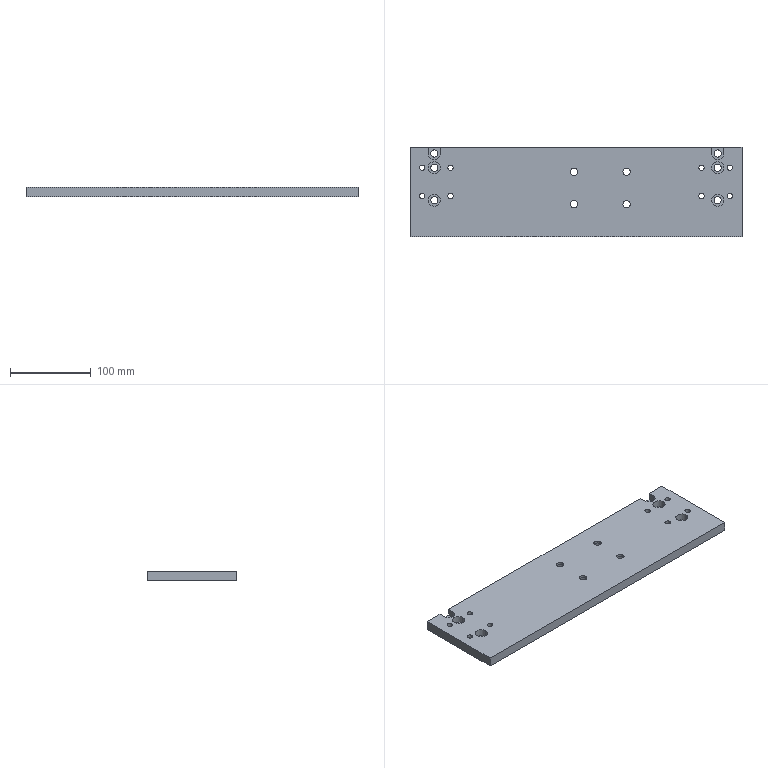Part | SolidWorks | features 3DProfileFeature 3, HoleWzd 3, ICE 2, LPattern 2, Extrusion 1 | 1 solid | 98 faces | box 410 x 110 x 12 mm | volume 516360 mm3 | cylinder 70 | plane 28 | commonest cylinder face diameters 9 x20 15 x18 6.6 x16 11 x16